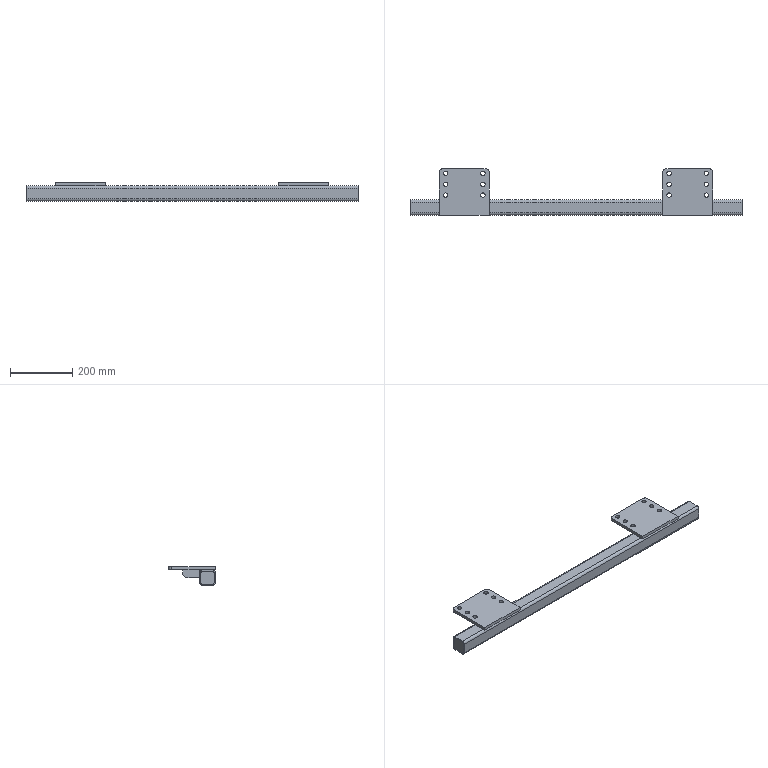Part | STEP file | REAR_AXIS_PROFILEV11_Default<Machined> | 9 solids | 106 faces | box 1070 x 150 x 60 mm | volume 1274604 mm3 | plane 62 | cylinder 44 | commonest cylinder face diameters 14 x24 8 x12 16 x4 20 x4